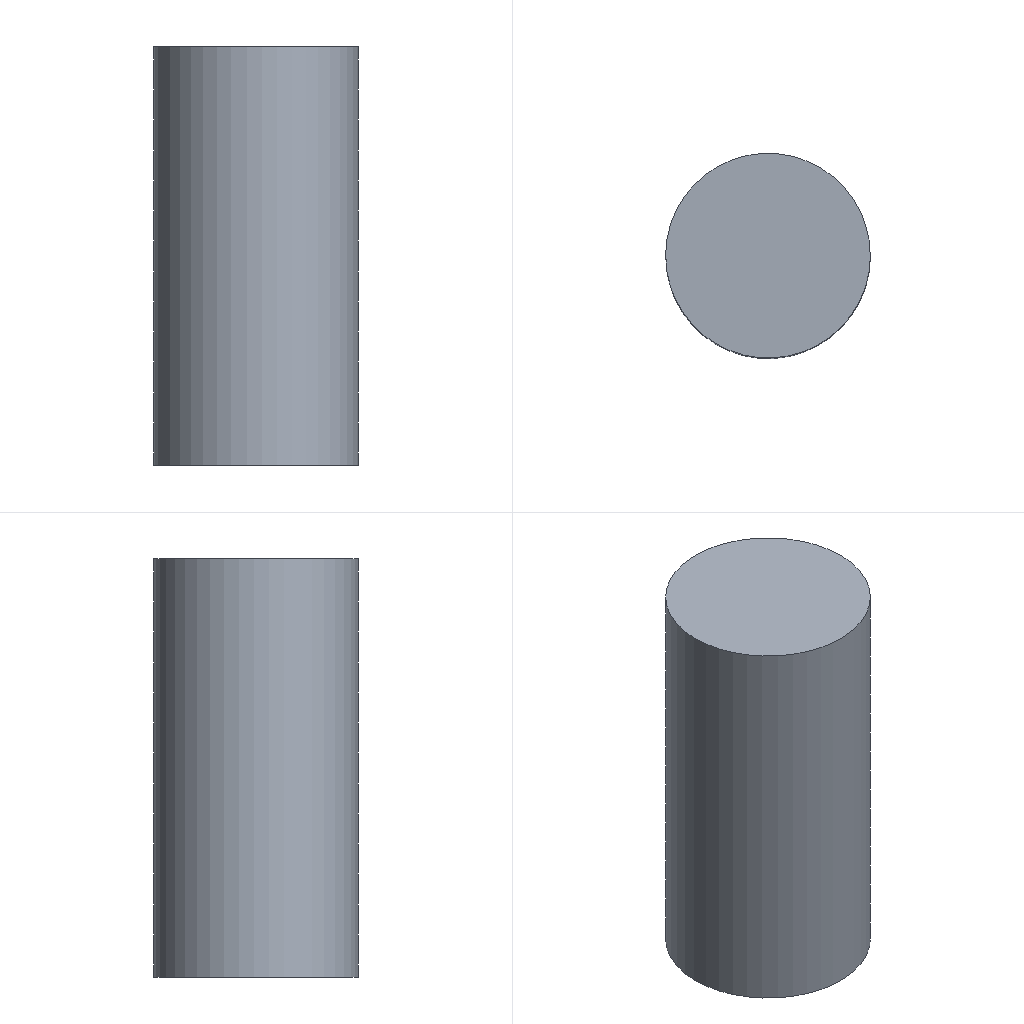Simulation study | abaqus
Set-up summary:
category,name,step,type,value,unit,region
solver,abaqus
solver,version,,,Abaqus/Standard 2020
units,not stated in the deck,,not stated
analysis,deck,,static,static
load_step,Step-1,Step-1,static
load_step,requested,,,1
mesh,nodes,,,29125
mesh,elements,,,72940
element_type,C3D4,,solid,67594
element_type,C3D8R,,solid,5346
load,load commands in deck,,count,2
bc,support commands in deck,,count,5
material,EPS,,in results
material,SOIL,,in results
check,setup vs results,,match,"per instance, exact: element labels, types and connectivity; labels of the nodes the elements use; coordinates of those nodes at SINGLE_PRECISION in 1 of 2 instance(s)"
Abaqus input file, long lists of numbers shortened, first 1042 of 4091 lines:
*Heading
** Job name: Job-1 Model name: Model-1
** Generated by: Abaqus/CAE 2020
*Preprint, echo=NO, model=NO, history=NO, contact=NO
**
** PARTS
**
*Part, name=Parricles
*Node
      1,    12.783,  0.9336,   23.451
      2,    13.63,   4.46,   20.722
** (22963 more lines like these left out)
*Element, type=C3D4
  1, 17460, 17461, 17462, 17463
  2,  2296, 17464, 17465, 17460
** (67592 more lines like these left out)
*Nset, nset=Set-4, generate
     1,  22965,      1
*Elset, elset=Set-4, generate
     1,  67594,      1
*Nset, nset=eps-all, generate
     1,  22965,      1
*Elset, elset=eps-all, generate
     1,  67594,      1
** Section: eps
*Solid Section, elset=Set-4, material=eps
,
*End Part
**
*Part, name=soil
*Node
      1,   15.958,  -11.294,           0.
      2,   18.578,  -6.089,           0.
** (6158 more lines like these left out)
*Element, type=C3D8R
   1,  291,  286,  263,  294,   71,   66,   43,   74
   2,  286,  260,  239,  263,   66,   40,   19,   43
** (5344 more lines like these left out)
*Nset, nset=Set-2, generate
    1,  6160,     1
*Elset, elset=Set-2, generate
    1,  5346,     1
** Section: soil
*Solid Section, elset=Set-2, material=soil
,
*End Part
**
**
** ASSEMBLY
**
*Assembly, name=Assembly
**
*Instance, name=Parricles-1, part=Parricles
       -14.6,        -14.7,           0.
*End Instance
**
*Instance, name=soil-1, part=soil
*End Instance
**
*Nset, nset=Set-1, instance=soil-1, generate
   1,  220,    1
*Elset, elset=Set-1, instance=soil-1, generate
   1,  198,    1
*Nset, nset=Set-2, instance=soil-1, generate
 5941,  6160,     1
*Elset, elset=Set-2, instance=soil-1, generate
 5149,  5346,     1
*Nset, nset=Set-3, instance=soil-1, generate
   1,  220,    1
*Elset, elset=Set-3, instance=soil-1, generate
   1,  198,    1
*Elset, elset=_Surf-1_S4, internal, instance=soil-1
    2,    3,    8,    9,   10,   15,   22,   23,   24,   31,   32,   36,   37,   39,   41,   43
   44,   61,   62,   85,   88,  186,  187,  200,  201,  206,  207,  208,  213,  220,  221,  222
** (37 more lines like these left out)
*Elset, elset=_Surf-1_S6, internal, instance=soil-1
    4,    5,    7,   11,   12,   13,   14,   17,   19,   21,   30,   35,   38,   40,   42,   49
   53,   56,   59,  202,  203,  205,  209,  210,  211,  212,  215,  217,  219,  228,  233,  236
** (31 more lines like these left out)
*Surface, type=ELEMENT, name=Surf-1
_Surf-1_S4, S4
_Surf-1_S6, S6
*Elset, elset=_Surf-2_S1, internal, instance=soil-1, generate
 5149,  5346,     1
*Surface, type=ELEMENT, name=Surf-2
_Surf-2_S1, S1
** Constraint: Constraint-1
*Embedded Element
Parricles-1.eps-all
*Elset, elset=__Int-1_gcs0_1_S4, internal, instance=Parricles-1
  11,  14,  23, 142
*Elset, elset=__Int-1_gcs0_1_S3, internal, instance=Parricles-1
  30,  39,  43,  47,  49,  50,  52,  62,  75,  77,  80,  85,  87,  88,  89,  90
  92,  93,  97,  98, 100, 101, 103, 104, 105, 106, 107, 108, 109, 110, 111, 112
** (2 more lines like these left out)
*Elset, elset=__Int-1_gcs0_1_S1, internal, instance=Parricles-1
 74,
*Elset, elset=__Int-1_gcs0_1_S2, internal, instance=Parricles-1
  86,  91,  96, 102, 141, 147
*Surface, type=ELEMENT, name=_Int-1_gcs0_1, internal
__Int-1_gcs0_1_S4, S4
__Int-1_gcs0_1_S3, S3
__Int-1_gcs0_1_S2, S2
__Int-1_gcs0_1_S1, S1
*Elset, elset=__Int-1_gcs0_2_S3, internal, instance=Parricles-1
 162, 187, 193, 196, 199, 200, 204, 213, 214, 215, 216, 217, 218, 219, 220, 222
 223, 226, 232, 233, 234, 236, 237, 238, 239, 241, 242, 243, 244, 245, 246, 247
** (2 more lines like these left out)
*Elset, elset=__Int-1_gcs0_2_S4, internal, instance=Parricles-1
 174, 212, 235, 255
*Elset, elset=__Int-1_gcs0_2_S1, internal, instance=Parricles-1
 224,
*Elset, elset=__Int-1_gcs0_2_S2, internal, instance=Parricles-1
 225, 227, 231, 260, 271, 284
*Surface, type=ELEMENT, name=_Int-1_gcs0_2, internal
__Int-1_gcs0_2_S3, S3
__Int-1_gcs0_2_S4, S4
__Int-1_gcs0_2_S2, S2
__Int-1_gcs0_2_S1, S1
*Elset, elset=__Int-1_gcs0_3_S3, internal, instance=Parricles-1
 304, 310, 322, 323, 328, 334, 340, 361, 362, 363, 365, 366, 367, 369, 370, 371
 375, 376, 377, 379, 380, 381, 382, 383, 384, 385, 387, 388, 389, 390, 391, 392
** (3 more lines like these left out)
*Elset, elset=__Int-1_gcs0_3_S2, internal, instance=Parricles-1
 306, 437
*Elset, elset=__Int-1_gcs0_3_S4, internal, instance=Parricles-1
 330,
*Elset, elset=__Int-1_gcs0_3_S1, internal, instance=Parricles-1
 431,
*Surface, type=ELEMENT, name=_Int-1_gcs0_3, internal
__Int-1_gcs0_3_S3, S3
__Int-1_gcs0_3_S2, S2
__Int-1_gcs0_3_S4, S4
__Int-1_gcs0_3_S1, S1
*Elset, elset=__Int-1_gcs0_4_S1, internal, instance=Parricles-1
 495, 524, 598
*Elset, elset=__Int-1_gcs0_4_S4, internal, instance=Parricles-1
 500, 502, 560, 586
*Elset, elset=__Int-1_gcs0_4_S3, internal, instance=Parricles-1
 509, 515, 530, 531, 532, 533, 535, 536, 537, 539, 542, 543, 544, 545, 546, 547
 548, 551, 552, 555, 556, 557, 558, 559, 561, 562, 563, 564, 566, 567, 569, 570
** (2 more lines like these left out)
*Elset, elset=__Int-1_gcs0_4_S2, internal, instance=Parricles-1
 550, 610
*Surface, type=ELEMENT, name=_Int-1_gcs0_4, internal
__Int-1_gcs0_4_S1, S1
__Int-1_gcs0_4_S4, S4
__Int-1_gcs0_4_S2, S2
__Int-1_gcs0_4_S3, S3
*Elset, elset=__Int-1_gcs0_5_S4, internal, instance=Parricles-1
 618, 633, 712
*Elset, elset=__Int-1_gcs0_5_S3, internal, instance=Parricles-1
 620, 623, 626, 644, 648, 666, 677, 679, 680, 681, 682, 683, 684, 685, 687, 689
 690, 691, 692, 693, 694, 695, 696, 697, 698, 699, 701, 702, 703, 704, 705, 708
** (2 more lines like these left out)
*Elset, elset=__Int-1_gcs0_5_S1, internal, instance=Parricles-1
 650,
*Elset, elset=__Int-1_gcs0_5_S2, internal, instance=Parricles-1
 678,
*Surface, type=ELEMENT, name=_Int-1_gcs0_5, internal
__Int-1_gcs0_5_S4, S4
__Int-1_gcs0_5_S3, S3
__Int-1_gcs0_5_S2, S2
__Int-1_gcs0_5_S1, S1
*Elset, elset=__Int-1_gcs0_6_S3, internal, instance=Parricles-1
 765, 770, 819, 823, 829, 832, 833, 834, 835, 837, 839, 840, 841, 842, 843, 846
 847, 850, 851, 852, 854, 856, 858, 859, 860, 861, 862, 863, 864, 865, 866, 868
** (2 more lines like these left out)
*Elset, elset=__Int-1_gcs0_6_S4, internal, instance=Parricles-1
 792, 826, 828, 838, 844, 867, 888, 902
*Elset, elset=__Int-1_gcs0_6_S1, internal, instance=Parricles-1
 796,
*Elset, elset=__Int-1_gcs0_6_S2, internal, instance=Parricles-1
 845, 896, 903
*Surface, type=ELEMENT, name=_Int-1_gcs0_6, internal
__Int-1_gcs0_6_S3, S3
__Int-1_gcs0_6_S4, S4
__Int-1_gcs0_6_S2, S2
__Int-1_gcs0_6_S1, S1
*Elset, elset=__Int-1_gcs0_7_S3, internal, instance=Parricles-1
  931,  962,  964,  985,  986,  987,  988,  989,  990,  991,  992,  993,  994,  996,  997, 1000
 1001, 1003, 1004, 1005, 1006, 1009, 1011, 1012, 1014, 1015, 1016, 1017, 1018, 1019, 1020, 1021
** (3 more lines like these left out)
*Elset, elset=__Int-1_gcs0_7_S4, internal, instance=Parricles-1
 954, 961
*Elset, elset=__Int-1_gcs0_7_S2, internal, instance=Parricles-1
  995, 1008, 1022, 1054
*Surface, type=ELEMENT, name=_Int-1_gcs0_7, internal
__Int-1_gcs0_7_S3, S3
__Int-1_gcs0_7_S4, S4
__Int-1_gcs0_7_S2, S2
*Elset, elset=__Int-1_gcs0_8_S3, internal, instance=Parricles-1
 1071, 1075, 1079, 1083, 1090, 1113, 1121, 1130, 1131, 1133, 1134, 1136, 1137, 1138, 1139, 1140
 1142, 1145, 1148, 1149, 1150, 1152, 1153, 1154, 1155, 1156, 1157, 1158, 1159, 1161, 1162, 1163
** (2 more lines like these left out)
*Elset, elset=__Int-1_gcs0_8_S2, internal, instance=Parricles-1
 1086, 1151, 1165
*Elset, elset=__Int-1_gcs0_8_S1, internal, instance=Parricles-1
 1116, 1166, 1182
*Elset, elset=__Int-1_gcs0_8_S4, internal, instance=Parricles-1
 1144, 1194
*Surface, type=ELEMENT, name=_Int-1_gcs0_8, internal
__Int-1_gcs0_8_S3, S3
__Int-1_gcs0_8_S2, S2
__Int-1_gcs0_8_S4, S4
__Int-1_gcs0_8_S1, S1
*Elset, elset=__Int-1_gcs0_9_S4, internal, instance=Parricles-1
 1217, 1300
*Elset, elset=__Int-1_gcs0_9_S3, internal, instance=Parricles-1
 1230, 1234, 1248, 1269, 1272, 1273, 1275, 1276, 1277, 1280, 1282, 1283, 1284, 1285, 1287, 1288
 1289, 1290, 1291, 1292, 1293, 1294, 1295, 1297, 1299, 1303, 1304, 1306, 1307, 1308, 1309, 1310
** (2 more lines like these left out)
*Elset, elset=__Int-1_gcs0_9_S2, internal, instance=Parricles-1
 1252, 1253, 1298, 1305, 1311, 1338
*Surface, type=ELEMENT, name=_Int-1_gcs0_9, internal
__Int-1_gcs0_9_S4, S4
__Int-1_gcs0_9_S3, S3
__Int-1_gcs0_9_S2, S2
*Elset, elset=__Int-1_gcs0_10_S3, internal, instance=Parricles-1
 1346, 1348, 1362, 1363, 1367, 1368, 1373, 1378, 1394, 1403, 1404, 1405, 1406, 1407, 1408, 1409
 1410, 1411, 1412, 1414, 1415, 1416, 1417, 1419, 1422, 1424, 1425, 1426, 1427, 1428, 1430, 1431
** (2 more lines like these left out)
*Elset, elset=__Int-1_gcs0_10_S1, internal, instance=Parricles-1
 1350, 1361, 1472
*Elset, elset=__Int-1_gcs0_10_S2, internal, instance=Parricles-1
 1351, 1354
*Elset, elset=__Int-1_gcs0_10_S4, internal, instance=Parricles-1
 1389, 1436, 1459
*Surface, type=ELEMENT, name=_Int-1_gcs0_10, internal
__Int-1_gcs0_10_S3, S3
__Int-1_gcs0_10_S1, S1
__Int-1_gcs0_10_S2, S2
__Int-1_gcs0_10_S4, S4
*Elset, elset=__Int-1_gcs0_11_S2, internal, instance=Parricles-1
 1479, 1544, 1568, 1603, 1605, 1608
*Elset, elset=__Int-1_gcs0_11_S3, internal, instance=Parricles-1
 1487, 1501, 1524, 1530, 1539, 1541, 1542, 1545, 1560, 1564, 1565, 1566, 1567, 1569, 1570, 1571
 1572, 1573, 1574, 1575, 1576, 1577, 1579, 1580, 1581, 1582, 1584, 1588, 1589, 1590, 1592, 1594
** (2 more lines like these left out)
*Elset, elset=__Int-1_gcs0_11_S1, internal, instance=Parricles-1
 1552,
*Elset, elset=__Int-1_gcs0_11_S4, internal, instance=Parricles-1
 1585, 1593
*Surface, type=ELEMENT, name=_Int-1_gcs0_11, internal
__Int-1_gcs0_11_S2, S2
__Int-1_gcs0_11_S3, S3
__Int-1_gcs0_11_S4, S4
__Int-1_gcs0_11_S1, S1
*Elset, elset=__Int-1_gcs0_12_S2, internal, instance=Parricles-1
 1637, 1703, 1733, 1735, 1750, 1762
*Elset, elset=__Int-1_gcs0_12_S3, internal, instance=Parricles-1
 1650, 1653, 1655, 1682, 1689, 1705, 1706, 1707, 1708, 1709, 1711, 1712, 1713, 1714, 1715, 1717
 1718, 1719, 1720, 1721, 1723, 1724, 1725, 1726, 1727, 1728, 1729, 1731, 1734, 1737, 1739, 1740
** (2 more lines like these left out)
*Elset, elset=__Int-1_gcs0_12_S1, internal, instance=Parricles-1
 1656, 1680
*Elset, elset=__Int-1_gcs0_12_S4, internal, instance=Parricles-1
 1688, 1704, 1730
*Surface, type=ELEMENT, name=_Int-1_gcs0_12, internal
__Int-1_gcs0_12_S2, S2
__Int-1_gcs0_12_S3, S3
__Int-1_gcs0_12_S4, S4
__Int-1_gcs0_12_S1, S1
*Elset, elset=__Int-1_gcs0_13_S2, internal, instance=Parricles-1
 1780, 1849, 1860, 1910, 1927
*Elset, elset=__Int-1_gcs0_13_S4, internal, instance=Parricles-1
 1784, 1796, 1822, 1867, 1887, 1903
*Elset, elset=__Int-1_gcs0_13_S3, internal, instance=Parricles-1
 1791, 1795, 1803, 1811, 1819, 1846, 1851, 1861, 1863, 1864, 1866, 1868, 1869, 1870, 1872, 1877
 1878, 1880, 1883, 1884, 1885, 1886, 1888, 1889, 1890, 1891, 1892, 1893, 1894, 1895, 1896, 1897
** (3 more lines like these left out)
*Surface, type=ELEMENT, name=_Int-1_gcs0_13, internal
__Int-1_gcs0_13_S2, S2
__Int-1_gcs0_13_S4, S4
__Int-1_gcs0_13_S3, S3
*Elset, elset=__Int-1_gcs0_14_S3, internal, instance=Parricles-1
 1947, 1955, 1973, 1975, 1980, 1991, 1997, 2007, 2028, 2032, 2033, 2034, 2035, 2036, 2037, 2039
 2041, 2042, 2043, 2044, 2045, 2050, 2051, 2052, 2055, 2056, 2057, 2058, 2059, 2060, 2062, 2064
** (2 more lines like these left out)
*Elset, elset=__Int-1_gcs0_14_S1, internal, instance=Parricles-1
 1953, 1956, 1958, 2002
*Elset, elset=__Int-1_gcs0_14_S4, internal, instance=Parricles-1
 1961, 1988, 2011, 2061
*Elset, elset=__Int-1_gcs0_14_S2, internal, instance=Parricles-1
 2017, 2084, 2085, 2100
*Surface, type=ELEMENT, name=_Int-1_gcs0_14, internal
__Int-1_gcs0_14_S3, S3
__Int-1_gcs0_14_S1, S1
__Int-1_gcs0_14_S4, S4
__Int-1_gcs0_14_S2, S2
*Elset, elset=__Int-1_gcs0_15_S4, internal, instance=Parricles-1
 2126, 2147
*Elset, elset=__Int-1_gcs0_15_S3, internal, instance=Parricles-1
 2135, 2144, 2145, 2151, 2164, 2170, 2172, 2174, 2178, 2180, 2181, 2182, 2183, 2184, 2185, 2188
 2189, 2190, 2191, 2194, 2195, 2196, 2197, 2198, 2199, 2200, 2201, 2202, 2203, 2204, 2205, 2206
** (2 more lines like these left out)
*Elset, elset=__Int-1_gcs0_15_S1, internal, instance=Parricles-1
 2161, 2166, 2235
*Elset, elset=__Int-1_gcs0_15_S2, internal, instance=Parricles-1
 2192, 2193, 2228, 2234, 2236
*Surface, type=ELEMENT, name=_Int-1_gcs0_15, internal
__Int-1_gcs0_15_S4, S4
__Int-1_gcs0_15_S3, S3
__Int-1_gcs0_15_S2, S2
__Int-1_gcs0_15_S1, S1
*Elset, elset=__Int-1_gcs0_16_S3, internal, instance=Parricles-1
 2249, 2258, 2269, 2298, 2305, 2309, 2311, 2313, 2315, 2316, 2317, 2318, 2319, 2321, 2322, 2323
 2324, 2327, 2328, 2329, 2330, 2332, 2333, 2334, 2335, 2337, 2338, 2339, 2341, 2342, 2343, 2344
** (2 more lines like these left out)
*Elset, elset=__Int-1_gcs0_16_S2, internal, instance=Parricles-1
 2250, 2314, 2340, 2350, 2354, 2356, 2369
*Elset, elset=__Int-1_gcs0_16_S4, internal, instance=Parricles-1
 2325, 2371
*Surface, type=ELEMENT, name=_Int-1_gcs0_16, internal
__Int-1_gcs0_16_S3, S3
__Int-1_gcs0_16_S2, S2
__Int-1_gcs0_16_S4, S4
*Elset, elset=__Int-1_gcs0_17_S3, internal, instance=Parricles-1
 2384, 2395, 2402, 2404, 2418, 2425, 2427, 2433, 2449, 2451, 2455, 2456, 2457, 2458, 2459, 2460
 2461, 2462, 2463, 2464, 2465, 2466, 2468, 2469, 2470, 2471, 2472, 2473, 2474, 2475, 2476, 2477
** (2 more lines like these left out)
*Elset, elset=__Int-1_gcs0_17_S4, internal, instance=Parricles-1
 2399, 2419, 2448, 2452
*Elset, elset=__Int-1_gcs0_17_S1, internal, instance=Parricles-1
 2420,
*Elset, elset=__Int-1_gcs0_17_S2, internal, instance=Parricles-1
 2453, 2491, 2508, 2511, 2517
*Surface, type=ELEMENT, name=_Int-1_gcs0_17, internal
__Int-1_gcs0_17_S3, S3
__Int-1_gcs0_17_S4, S4
__Int-1_gcs0_17_S2, S2
__Int-1_gcs0_17_S1, S1
*Elset, elset=__Int-1_gcs0_18_S3, internal, instance=Parricles-1
 2533, 2568, 2569, 2576, 2578, 2579, 2580, 2582, 2583, 2588, 2590, 2591, 2593, 2594, 2596, 2597
 2600, 2601, 2602, 2603, 2605, 2606, 2607, 2608, 2609, 2611, 2612, 2614, 2615, 2616, 2617, 2618
** (2 more lines like these left out)
*Elset, elset=__Int-1_gcs0_18_S1, internal, instance=Parricles-1
 2541, 2560, 2563
*Elset, elset=__Int-1_gcs0_18_S2, internal, instance=Parricles-1
 2543, 2565, 2585, 2640, 2641, 2643
*Elset, elset=__Int-1_gcs0_18_S4, internal, instance=Parricles-1
 2573, 2598, 2613, 2620
*Surface, type=ELEMENT, name=_Int-1_gcs0_18, internal
__Int-1_gcs0_18_S3, S3
__Int-1_gcs0_18_S1, S1
__Int-1_gcs0_18_S2, S2
__Int-1_gcs0_18_S4, S4
*Elset, elset=__Int-1_gcs0_19_S3, internal, instance=Parricles-1
 2664, 2666, 2669, 2684, 2691, 2695, 2696, 2697, 2698, 2699, 2700, 2701, 2702, 2703, 2704, 2708
 2709, 2711, 2712, 2714, 2715, 2716, 2717, 2718, 2720, 2721, 2722, 2723, 2724, 2726, 2727, 2728
** (3 more lines like these left out)
*Elset, elset=__Int-1_gcs0_19_S4, internal, instance=Parricles-1
 2671,
*Elset, elset=__Int-1_gcs0_19_S2, internal, instance=Parricles-1
 2705, 2732
*Surface, type=ELEMENT, name=_Int-1_gcs0_19, internal
__Int-1_gcs0_19_S3, S3
__Int-1_gcs0_19_S4, S4
__Int-1_gcs0_19_S2, S2
*Elset, elset=__Int-1_gcs0_20_S4, internal, instance=Parricles-1
 2788, 2812, 2838
*Elset, elset=__Int-1_gcs0_20_S3, internal, instance=Parricles-1
 2796, 2823, 2848, 2860, 2875, 2877, 2878, 2879, 2880, 2881, 2884, 2885, 2887, 2889, 2890, 2891
 2893, 2895, 2896, 2897, 2898, 2899, 2900, 2901, 2903, 2904, 2905, 2906, 2907, 2908, 2910, 2911
** (3 more lines like these left out)
*Elset, elset=__Int-1_gcs0_20_S2, internal, instance=Parricles-1
 2902,
*Surface, type=ELEMENT, name=_Int-1_gcs0_20, internal
__Int-1_gcs0_20_S4, S4
__Int-1_gcs0_20_S3, S3
__Int-1_gcs0_20_S2, S2
*Elset, elset=__Int-1_gcs0_21_S1, internal, instance=Parricles-1
 2964, 2984
*Elset, elset=__Int-1_gcs0_21_S3, internal, instance=Parricles-1
 2967, 2970, 2980, 2983, 2987, 2995, 3012, 3013, 3042, 3047, 3048, 3049, 3050, 3051, 3052, 3053
 3054, 3055, 3056, 3058, 3060, 3062, 3063, 3065, 3067, 3068, 3069, 3070, 3071, 3072, 3073, 3074
** (3 more lines like these left out)
*Elset, elset=__Int-1_gcs0_21_S4, internal, instance=Parricles-1
 3008, 3080
*Elset, elset=__Int-1_gcs0_21_S2, internal, instance=Parricles-1
 3057, 3103
*Surface, type=ELEMENT, name=_Int-1_gcs0_21, internal
__Int-1_gcs0_21_S1, S1
__Int-1_gcs0_21_S3, S3
__Int-1_gcs0_21_S4, S4
__Int-1_gcs0_21_S2, S2
*Elset, elset=__Int-1_gcs0_22_S3, internal, instance=Parricles-1
 3126, 3146, 3149, 3151, 3168, 3170, 3171, 3180, 3184, 3195, 3196, 3197, 3199, 3202, 3205, 3206
 3207, 3208, 3211, 3212, 3214, 3215, 3216, 3217, 3219, 3220, 3221, 3222, 3223, 3224, 3225, 3227
** (2 more lines like these left out)
*Elset, elset=__Int-1_gcs0_22_S4, internal, instance=Parricles-1
 3135, 3159, 3172, 3204, 3251, 3260
*Elset, elset=__Int-1_gcs0_22_S2, internal, instance=Parricles-1
 3189, 3198, 3210, 3231
*Surface, type=ELEMENT, name=_Int-1_gcs0_22, internal
__Int-1_gcs0_22_S3, S3
__Int-1_gcs0_22_S4, S4
__Int-1_gcs0_22_S2, S2
*Elset, elset=__Int-1_gcs0_23_S4, internal, instance=Parricles-1
 3271, 3284, 3294
*Elset, elset=__Int-1_gcs0_23_S3, internal, instance=Parricles-1
 3285, 3290, 3295, 3301, 3314, 3316, 3319, 3320, 3322, 3323, 3324, 3325, 3326, 3327, 3328, 3329
 3330, 3331, 3332, 3333, 3334, 3336, 3337, 3338, 3339, 3340, 3342, 3343, 3344, 3345, 3347, 3348
** (3 more lines like these left out)
*Elset, elset=__Int-1_gcs0_23_S2, internal, instance=Parricles-1
 3371, 3382, 3384
*Elset, elset=__Int-1_gcs0_23_S1, internal, instance=Parricles-1
 3376,
*Surface, type=ELEMENT, name=_Int-1_gcs0_23, internal
__Int-1_gcs0_23_S4, S4
__Int-1_gcs0_23_S3, S3
__Int-1_gcs0_23_S2, S2
__Int-1_gcs0_23_S1, S1
*Elset, elset=__Int-1_gcs0_24_S3, internal, instance=Parricles-1
 3394, 3409, 3421, 3432, 3436, 3443, 3444, 3445, 3446, 3448, 3450, 3451, 3455, 3456, 3457, 3458
 3459, 3460, 3461, 3462, 3464, 3465, 3466, 3467, 3468, 3469, 3470, 3471, 3473, 3474, 3475, 3476
** (2 more lines like these left out)
*Elset, elset=__Int-1_gcs0_24_S4, internal, instance=Parricles-1
 3399, 3425, 3447
*Elset, elset=__Int-1_gcs0_24_S1, internal, instance=Parricles-1
 3430,
*Elset, elset=__Int-1_gcs0_24_S2, internal, instance=Parricles-1
 3449, 3472, 3492
*Surface, type=ELEMENT, name=_Int-1_gcs0_24, internal
__Int-1_gcs0_24_S3, S3
__Int-1_gcs0_24_S4, S4
__Int-1_gcs0_24_S2, S2
__Int-1_gcs0_24_S1, S1
*Elset, elset=__Int-1_gcs0_25_S3, internal, instance=Parricles-1
 3525, 3553, 3556, 3567, 3569, 3570, 3571, 3573, 3574, 3575, 3576, 3577, 3578, 3580, 3582, 3583
 3584, 3585, 3586, 3588, 3589, 3590, 3591, 3592, 3593, 3594, 3595, 3596, 3598, 3599, 3600, 3601
** (3 more lines like these left out)
*Elset, elset=__Int-1_gcs0_25_S4, internal, instance=Parricles-1
 3529, 3536, 3572
*Elset, elset=__Int-1_gcs0_25_S2, internal, instance=Parricles-1
 3579, 3581, 3587, 3613
*Surface, type=ELEMENT, name=_Int-1_gcs0_25, internal
__Int-1_gcs0_25_S3, S3
__Int-1_gcs0_25_S4, S4
__Int-1_gcs0_25_S2, S2
*Elset, elset=__Int-1_gcs0_26_S1, internal, instance=Parricles-1
 3644, 3679
*Elset, elset=__Int-1_gcs0_26_S3, internal, instance=Parricles-1
 3654, 3664, 3666, 3672, 3688, 3690, 3693, 3699, 3700, 3702, 3703, 3704, 3706, 3707, 3708, 3710
 3711, 3716, 3717, 3718, 3723, 3725, 3728, 3730, 3731, 3734, 3735, 3736, 3737, 3738, 3739, 3741
** (2 more lines like these left out)
*Elset, elset=__Int-1_gcs0_26_S4, internal, instance=Parricles-1
 3659, 3674, 3677, 3685, 3713
*Elset, elset=__Int-1_gcs0_26_S2, internal, instance=Parricles-1
 3712, 3715, 3733, 3744, 3755, 3768
*Surface, type=ELEMENT, name=_Int-1_gcs0_26, internal
__Int-1_gcs0_26_S1, S1
__Int-1_gcs0_26_S3, S3
__Int-1_gcs0_26_S4, S4
__Int-1_gcs0_26_S2, S2
*Elset, elset=__Int-1_gcs0_27_S3, internal, instance=Parricles-1
 3782, 3785, 3843, 3844, 3849, 3857, 3858, 3859, 3860, 3861, 3862, 3863, 3864, 3866, 3867, 3868
 3869, 3871, 3874, 3875, 3877, 3878, 3879, 3880, 3882, 3883, 3885, 3886, 3887, 3891, 3892, 3893
** (3 more lines like these left out)
*Elset, elset=__Int-1_gcs0_27_S4, internal, instance=Parricles-1
 3784, 3827, 3926, 3940
*Elset, elset=__Int-1_gcs0_27_S2, internal, instance=Parricles-1
 3870, 3888, 3902
*Surface, type=ELEMENT, name=_Int-1_gcs0_27, internal
__Int-1_gcs0_27_S3, S3
__Int-1_gcs0_27_S4, S4
__Int-1_gcs0_27_S2, S2
*Elset, elset=__Int-1_gcs0_28_S3, internal, instance=Parricles-1
 3944, 3970, 3977, 3995, 4012, 4013, 4014, 4015, 4016, 4017, 4018, 4019, 4020, 4022, 4023, 4026
 4027, 4028, 4029, 4030, 4031, 4032, 4033, 4034, 4035, 4037, 4038, 4039, 4040, 4041, 4042, 4043
** (2 more lines like these left out)
*Elset, elset=__Int-1_gcs0_28_S4, internal, instance=Parricles-1
 3954,
*Elset, elset=__Int-1_gcs0_28_S1, internal, instance=Parricles-1
 3967, 3978, 3979, 3980, 3984
*Elset, elset=__Int-1_gcs0_28_S2, internal, instance=Parricles-1
 4024, 4025, 4036, 4051, 4069
*Surface, type=ELEMENT, name=_Int-1_gcs0_28, internal
__Int-1_gcs0_28_S3, S3
__Int-1_gcs0_28_S4, S4
__Int-1_gcs0_28_S2, S2
__Int-1_gcs0_28_S1, S1
*Elset, elset=__Int-1_gcs0_29_S4, internal, instance=Parricles-1
 4088, 4108, 4115, 4124, 4157, 4171, 4194
*Elset, elset=__Int-1_gcs0_29_S3, internal, instance=Parricles-1
 4092, 4100, 4114, 4131, 4133, 4147, 4151, 4153, 4154, 4155, 4156, 4163, 4164, 4168, 4170, 4173
 4174, 4175, 4176, 4177, 4178, 4179, 4182, 4185, 4186, 4188, 4189, 4190, 4191, 4192, 4193, 4195
** (2 more lines like these left out)
*Elset, elset=__Int-1_gcs0_29_S1, internal, instance=Parricles-1
 4134, 4169
*Elset, elset=__Int-1_gcs0_29_S2, internal, instance=Parricles-1
 4160, 4184, 4219, 4229
*Surface, type=ELEMENT, name=_Int-1_gcs0_29, internal
__Int-1_gcs0_29_S4, S4
__Int-1_gcs0_29_S3, S3
__Int-1_gcs0_29_S2, S2
__Int-1_gcs0_29_S1, S1
*Elset, elset=__Int-1_gcs0_30_S4, internal, instance=Parricles-1
 4233, 4241, 4273
*Elset, elset=__Int-1_gcs0_30_S3, internal, instance=Parricles-1
 4238, 4263, 4266, 4289, 4300, 4301, 4302, 4303, 4304, 4305, 4306, 4307, 4308, 4309, 4310, 4311
 4314, 4315, 4316, 4318, 4319, 4321, 4322, 4324, 4325, 4327, 4328, 4329, 4330, 4331, 4332, 4333
** (3 more lines like these left out)
*Elset, elset=__Int-1_gcs0_30_S1, internal, instance=Parricles-1
 4269,
*Elset, elset=__Int-1_gcs0_30_S2, internal, instance=Parricles-1
 4297, 4352
*Surface, type=ELEMENT, name=_Int-1_gcs0_30, internal
__Int-1_gcs0_30_S4, S4
__Int-1_gcs0_30_S3, S3
__Int-1_gcs0_30_S2, S2
__Int-1_gcs0_30_S1, S1
*Elset, elset=__Int-1_gcs0_31_S3, internal, instance=Parricles-1
 4385, 4403, 4413, 4419, 4433, 4434, 4439, 4449, 4451, 4467, 4469, 4470, 4471, 4472, 4473, 4474
 4476, 4478, 4479, 4480, 4481, 4482, 4483, 4484, 4485, 4486, 4488, 4489, 4491, 4495, 4496, 4497
** (2 more lines like these left out)
*Elset, elset=__Int-1_gcs0_31_S1, internal, instance=Parricles-1
 4396,
*Elset, elset=__Int-1_gcs0_31_S4, internal, instance=Parricles-1
 4414, 4465, 4492, 4501
*Elset, elset=__Int-1_gcs0_31_S2, internal, instance=Parricles-1
 4468, 4475, 4487, 4490, 4517
*Surface, type=ELEMENT, name=_Int-1_gcs0_31, internal
__Int-1_gcs0_31_S3, S3
__Int-1_gcs0_31_S1, S1
__Int-1_gcs0_31_S4, S4
__Int-1_gcs0_31_S2, S2
*Elset, elset=__Int-1_gcs0_32_S3, internal, instance=Parricles-1
 4552, 4553, 4574, 4579, 4581, 4605, 4606, 4608, 4610, 4611, 4612, 4613, 4615, 4616, 4619, 4622
 4623, 4624, 4625, 4626, 4627, 4628, 4629, 4630, 4631, 4633, 4634, 4635, 4636, 4638, 4639, 4640
** (3 more lines like these left out)
*Elset, elset=__Int-1_gcs0_32_S4, internal, instance=Parricles-1
 4557,
*Elset, elset=__Int-1_gcs0_32_S1, internal, instance=Parricles-1
 4587, 4658
*Elset, elset=__Int-1_gcs0_32_S2, internal, instance=Parricles-1
 4632, 4662
*Surface, type=ELEMENT, name=_Int-1_gcs0_32, internal
__Int-1_gcs0_32_S3, S3
__Int-1_gcs0_32_S4, S4
__Int-1_gcs0_32_S2, S2
__Int-1_gcs0_32_S1, S1
*Elset, elset=__Int-1_gcs0_33_S3, internal, instance=Parricles-1
 4696, 4714, 4720, 4739, 4758, 4759, 4760, 4763, 4766, 4767, 4769, 4771, 4773, 4774, 4775, 4776
 4778, 4779, 4781, 4783, 4784, 4785, 4787, 4788, 4791, 4792, 4793, 4794, 4795, 4796, 4798, 4800
** (3 more lines like these left out)
*Elset, elset=__Int-1_gcs0_33_S4, internal, instance=Parricles-1
 4699, 4733, 4742
*Elset, elset=__Int-1_gcs0_33_S2, internal, instance=Parricles-1
 4740, 4762, 4764, 4772, 4786, 4809
*Elset, elset=__Int-1_gcs0_33_S1, internal, instance=Parricles-1
 4741, 4805
*Surface, type=ELEMENT, name=_Int-1_gcs0_33, internal
__Int-1_gcs0_33_S3, S3
__Int-1_gcs0_33_S4, S4
__Int-1_gcs0_33_S2, S2
__Int-1_gcs0_33_S1, S1
*Elset, elset=__Int-1_gcs0_34_S4, internal, instance=Parricles-1
 4853, 4855, 4873, 4887, 4901, 4927, 4976, 4982
*Elset, elset=__Int-1_gcs0_34_S3, internal, instance=Parricles-1
 4899, 4906, 4907, 4908, 4909, 4910, 4911, 4913, 4914, 4915, 4916, 4917, 4918, 4919, 4920, 4922
 4923, 4924, 4925, 4926, 4928, 4930, 4931, 4934, 4935, 4937, 4938, 4939, 4942, 4944, 4945, 4947
** (2 more lines like these left out)
*Elset, elset=__Int-1_gcs0_34_S2, internal, instance=Parricles-1
 4941,
*Surface, type=ELEMENT, name=_Int-1_gcs0_34, internal
__Int-1_gcs0_34_S4, S4
__Int-1_gcs0_34_S3, S3
__Int-1_gcs0_34_S2, S2
*Elset, elset=__Int-1_gcs0_35_S4, internal, instance=Parricles-1
 4991, 5030, 5078, 5090, 5118
*Elset, elset=__Int-1_gcs0_35_S1, internal, instance=Parricles-1
 4998, 5108
*Elset, elset=__Int-1_gcs0_35_S3, internal, instance=Parricles-1
 4999, 5015, 5035, 5052, 5054, 5055, 5056, 5058, 5059, 5061, 5062, 5063, 5064, 5065, 5067, 5068
 5069, 5070, 5071, 5072, 5073, 5076, 5079, 5080, 5081, 5082, 5085, 5086, 5087, 5088, 5089, 5093
** (3 more lines like these left out)
*Elset, elset=__Int-1_gcs0_35_S2, internal, instance=Parricles-1
 5092,
*Surface, type=ELEMENT, name=_Int-1_gcs0_35, internal
__Int-1_gcs0_35_S4, S4
__Int-1_gcs0_35_S1, S1
__Int-1_gcs0_35_S2, S2
__Int-1_gcs0_35_S3, S3
*Elset, elset=__Int-1_gcs0_36_S3, internal, instance=Parricles-1
 5148, 5156, 5157, 5170, 5174, 5180, 5182, 5188, 5208, 5210, 5211, 5213, 5232, 5233, 5234, 5235
 5236, 5237, 5238, 5239, 5240, 5241, 5242, 5243, 5244, 5246, 5247, 5248, 5249, 5250, 5251, 5253
** (2 more lines like these left out)
*Elset, elset=__Int-1_gcs0_36_S4, internal, instance=Parricles-1
 5153, 5155, 5194, 5258, 5261, 5291, 5292
*Elset, elset=__Int-1_gcs0_36_S2, internal, instance=Parricles-1
 5163, 5259, 5277
*Elset, elset=__Int-1_gcs0_36_S1, internal, instance=Parricles-1
 5175, 5299
*Surface, type=ELEMENT, name=_Int-1_gcs0_36, internal
__Int-1_gcs0_36_S3, S3
__Int-1_gcs0_36_S4, S4
__Int-1_gcs0_36_S2, S2
__Int-1_gcs0_36_S1, S1
*Elset, elset=__Int-1_gcs0_37_S4, internal, instance=Parricles-1
 5302, 5305, 5324, 5338, 5357, 5403
*Elset, elset=__Int-1_gcs0_37_S3, internal, instance=Parricles-1
 5308, 5319, 5330, 5333, 5361, 5364, 5365, 5367, 5369, 5370, 5371, 5372, 5374, 5375, 5376, 5378
 5379, 5380, 5381, 5382, 5383, 5385, 5386, 5387, 5388, 5389, 5390, 5391, 5393, 5394, 5396, 5397
** (2 more lines like these left out)
*Elset, elset=__Int-1_gcs0_37_S1, internal, instance=Parricles-1
 5316,
*Elset, elset=__Int-1_gcs0_37_S2, internal, instance=Parricles-1
 5423,
*Surface, type=ELEMENT, name=_Int-1_gcs0_37, internal
__Int-1_gcs0_37_S4, S4
__Int-1_gcs0_37_S3, S3
__Int-1_gcs0_37_S2, S2
__Int-1_gcs0_37_S1, S1
*Elset, elset=__Int-1_gcs0_38_S3, internal, instance=Parricles-1
 5447, 5473, 5478, 5481, 5493, 5494, 5495, 5509, 5510, 5511, 5513, 5514, 5516, 5517, 5518, 5519
 5522, 5523, 5524, 5525, 5526, 5527, 5530, 5531, 5532, 5534, 5535, 5536, 5537, 5538, 5539, 5541
** (2 more lines like these left out)
*Elset, elset=__Int-1_gcs0_38_S2, internal, instance=Parricles-1
 5461, 5512, 5549, 5554
*Elset, elset=__Int-1_gcs0_38_S4, internal, instance=Parricles-1
 5501, 5506, 5521, 5569
*Surface, type=ELEMENT, name=_Int-1_gcs0_38, internal
__Int-1_gcs0_38_S3, S3
__Int-1_gcs0_38_S2, S2
__Int-1_gcs0_38_S4, S4
*Elset, elset=__Int-1_gcs0_39_S1, internal, instance=Parricles-1
 5580, 5591, 5592, 5598, 5631
*Elset, elset=__Int-1_gcs0_39_S3, internal, instance=Parricles-1
 5583, 5586, 5593, 5594, 5614, 5629, 5638, 5639, 5640, 5641, 5642, 5644, 5645, 5646, 5647, 5648
 5651, 5652, 5654, 5655, 5656, 5657, 5658, 5659, 5660, 5662, 5663, 5664, 5666, 5668, 5670, 5671
** (2 more lines like these left out)
*Elset, elset=__Int-1_gcs0_39_S4, internal, instance=Parricles-1
 5605, 5609, 5611, 5711
*Elset, elset=__Int-1_gcs0_39_S2, internal, instance=Parricles-1
 5709,
*Surface, type=ELEMENT, name=_Int-1_gcs0_39, internal
__Int-1_gcs0_39_S1, S1
__Int-1_gcs0_39_S3, S3
__Int-1_gcs0_39_S4, S4
__Int-1_gcs0_39_S2, S2
*Elset, elset=__Int-1_gcs0_40_S3, internal, instance=Parricles-1
 5720, 5726, 5734, 5742, 5777, 5782, 5788, 5794, 5795, 5796, 5798, 5799, 5800, 5802, 5803, 5804
 5805, 5807, 5808, 5809, 5811, 5812, 5813, 5814, 5816, 5817, 5818, 5820, 5822, 5824, 5825, 5826
** (2 more lines like these left out)
*Elset, elset=__Int-1_gcs0_40_S1, internal, instance=Parricles-1
 5730,
*Elset, elset=__Int-1_gcs0_40_S2, internal, instance=Parricles-1
 5750, 5806, 5863
*Elset, elset=__Int-1_gcs0_40_S4, internal, instance=Parricles-1
 5756, 5767, 5776, 5861
*Surface, type=ELEMENT, name=_Int-1_gcs0_40, internal
__Int-1_gcs0_40_S3, S3
__Int-1_gcs0_40_S1, S1
__Int-1_gcs0_40_S2, S2
__Int-1_gcs0_40_S4, S4
*Elset, elset=__Int-1_gcs0_41_S3, internal, instance=Parricles-1
 5885, 5890, 5897, 5899, 5932, 5933, 5936, 5937, 5938, 5939, 5940, 5941, 5943, 5944, 5946, 5947
 5948, 5949, 5950, 5953, 5954, 5955, 5956, 5958, 5959, 5960, 5961, 5962, 5963, 5964, 5965, 5966
** (2 more lines like these left out)
*Elset, elset=__Int-1_gcs0_41_S4, internal, instance=Parricles-1
 5902, 5925, 5942
*Elset, elset=__Int-1_gcs0_41_S2, internal, instance=Parricles-1
 5935, 5952, 5990
*Surface, type=ELEMENT, name=_Int-1_gcs0_41, internal
__Int-1_gcs0_41_S3, S3
__Int-1_gcs0_41_S4, S4
__Int-1_gcs0_41_S2, S2
*Elset, elset=__Int-1_gcs0_42_S1, internal, instance=Parricles-1
 6012, 6110
*Elset, elset=__Int-1_gcs0_42_S3, internal, instance=Parricles-1
 6026, 6051, 6053, 6056, 6057, 6058, 6059, 6060, 6061, 6062, 6063, 6064, 6065, 6066, 6067, 6068
 6070, 6072, 6073, 6074, 6076, 6077, 6078, 6079, 6082, 6083, 6084, 6085, 6086, 6088, 6090, 6091
** (3 more lines like these left out)
*Elset, elset=__Int-1_gcs0_42_S4, internal, instance=Parricles-1
 6052, 6097, 6131
*Elset, elset=__Int-1_gcs0_42_S2, internal, instance=Parricles-1
 6111,
*Surface, type=ELEMENT, name=_Int-1_gcs0_42, internal
__Int-1_gcs0_42_S1, S1
__Int-1_gcs0_42_S3, S3
__Int-1_gcs0_42_S4, S4
__Int-1_gcs0_42_S2, S2
*Elset, elset=__Int-1_gcs0_43_S4, internal, instance=Parricles-1
 6158, 6175, 6199, 6223, 6282
*Elset, elset=__Int-1_gcs0_43_S3, internal, instance=Parricles-1
 6161, 6188, 6190, 6205, 6208, 6209, 6211, 6212, 6213, 6214, 6215, 6216, 6217, 6218, 6219, 6221
 6222, 6224, 6225, 6226, 6227, 6228, 6230, 6231, 6232, 6235, 6237, 6238, 6240, 6241, 6242, 6243
** (2 more lines like these left out)
*Elset, elset=__Int-1_gcs0_43_S1, internal, instance=Parricles-1
 6165, 6169
*Elset, elset=__Int-1_gcs0_43_S2, internal, instance=Parricles-1
 6236, 6248, 6273
*Surface, type=ELEMENT, name=_Int-1_gcs0_43, internal
__Int-1_gcs0_43_S4, S4
__Int-1_gcs0_43_S3, S3
__Int-1_gcs0_43_S2, S2
__Int-1_gcs0_43_S1, S1
*Elset, elset=__Int-1_gcs0_44_S4, internal, instance=Parricles-1
 6291, 6346, 6391
*Elset, elset=__Int-1_gcs0_44_S3, internal, instance=Parricles-1
 6313, 6328, 6329, 6339, 6340, 6341, 6342, 6343, 6344, 6345, 6347, 6348, 6349, 6350, 6351, 6352
 6353, 6354, 6356, 6357, 6358, 6359, 6360, 6361, 6362, 6363, 6364, 6366, 6367, 6368, 6370, 6371
** (2 more lines like these left out)
*Elset, elset=__Int-1_gcs0_44_S2, internal, instance=Parricles-1
 6369, 6409, 6410
*Surface, type=ELEMENT, name=_Int-1_gcs0_44, internal
__Int-1_gcs0_44_S4, S4
__Int-1_gcs0_44_S3, S3
__Int-1_gcs0_44_S2, S2
*Elset, elset=__Int-1_gcs0_45_S3, internal, instance=Parricles-1
 6422, 6426, 6453, 6458, 6467, 6479, 6487, 6488, 6491, 6499, 6500, 6501, 6502, 6504, 6505, 6507
 6508, 6509, 6511, 6512, 6513, 6514, 6515, 6516, 6517, 6518, 6520, 6521, 6522, 6523, 6524, 6526
** (3 more lines like these left out)
*Elset, elset=__Int-1_gcs0_45_S1, internal, instance=Parricles-1
 6427, 6462
*Elset, elset=__Int-1_gcs0_45_S4, internal, instance=Parricles-1
 6436, 6459, 6503, 6525
*Elset, elset=__Int-1_gcs0_45_S2, internal, instance=Parricles-1
 6506, 6545
*Surface, type=ELEMENT, name=_Int-1_gcs0_45, internal
__Int-1_gcs0_45_S3, S3
__Int-1_gcs0_45_S1, S1
__Int-1_gcs0_45_S4, S4
__Int-1_gcs0_45_S2, S2
*Elset, elset=__Int-1_gcs0_46_S4, internal, instance=Parricles-1
 6583, 6628, 6644, 6649, 6674
*Elset, elset=__Int-1_gcs0_46_S3, internal, instance=Parricles-1
 6585, 6587, 6610, 6615, 6645, 6652, 6657, 6664, 6665, 6666, 6668, 6669, 6670, 6671, 6672, 6673
 6676, 6677, 6679, 6682, 6683, 6688, 6689, 6690, 6691, 6692, 6693, 6694, 6695, 6697, 6698, 6699
** (2 more lines like these left out)
*Elset, elset=__Int-1_gcs0_46_S1, internal, instance=Parricles-1
 6607, 6619, 6712
*Elset, elset=__Int-1_gcs0_46_S2, internal, instance=Parricles-1
 6633, 6661
*Surface, type=ELEMENT, name=_Int-1_gcs0_46, internal
__Int-1_gcs0_46_S4, S4
__Int-1_gcs0_46_S3, S3
__Int-1_gcs0_46_S2, S2
__Int-1_gcs0_46_S1, S1
*Elset, elset=__Int-1_gcs0_47_S3, internal, instance=Parricles-1
 6741, 6746, 6749, 6755, 6759, 6760, 6764, 6775, 6780, 6790, 6794, 6796, 6797, 6798, 6799, 6800
 6801, 6802, 6803, 6805, 6806, 6808, 6811, 6813, 6815, 6816, 6820, 6821, 6822, 6823, 6824, 6825
** (2 more lines like these left out)
*Elset, elset=__Int-1_gcs0_47_S1, internal, instance=Parricles-1
 6752, 6757, 6772, 6819, 6837
*Elset, elset=__Int-1_gcs0_47_S4, internal, instance=Parricles-1
 6804, 6814
*Elset, elset=__Int-1_gcs0_47_S2, internal, instance=Parricles-1
 6817, 6841, 6850, 6860, 6872
*Surface, type=ELEMENT, name=_Int-1_gcs0_47, internal
__Int-1_gcs0_47_S3, S3
__Int-1_gcs0_47_S1, S1
__Int-1_gcs0_47_S4, S4
__Int-1_gcs0_47_S2, S2
*Elset, elset=__Int-1_gcs0_48_S3, internal, instance=Parricles-1
 6880, 6891, 6894, 6931, 6932, 6935, 6942, 6943, 6946, 6947, 6948, 6954, 6955, 6956, 6957, 6959
 6960, 6962, 6964, 6967, 6968, 6969, 6970, 6975, 6976, 6977, 6978, 6979, 6980, 6981, 6982, 6983
** (3 more lines like these left out)
*Elset, elset=__Int-1_gcs0_48_S1, internal, instance=Parricles-1
 6892, 6938
*Elset, elset=__Int-1_gcs0_48_S4, internal, instance=Parricles-1
 6917, 7031
*Elset, elset=__Int-1_gcs0_48_S2, internal, instance=Parricles-1
 6945, 6953, 6990
*Surface, type=ELEMENT, name=_Int-1_gcs0_48, internal
__Int-1_gcs0_48_S3, S3
__Int-1_gcs0_48_S1, S1
__Int-1_gcs0_48_S4, S4
__Int-1_gcs0_48_S2, S2
*Elset, elset=__Int-1_gcs0_49_S3, internal, instance=Parricles-1
 7044, 7063, 7092, 7093, 7094, 7095, 7096, 7097, 7098, 7100, 7101, 7102, 7103, 7105, 7106, 7110
 7111, 7112, 7114, 7115, 7116, 7117, 7118, 7119, 7120, 7121, 7123, 7124, 7125, 7126, 7127, 7128
** (3 more lines like these left out)
*Elset, elset=__Int-1_gcs0_49_S4, internal, instance=Parricles-1
 7051, 7054, 7113
*Elset, elset=__Int-1_gcs0_49_S1, internal, instance=Parricles-1
 7062, 7074
*Elset, elset=__Int-1_gcs0_49_S2, internal, instance=Parricles-1
 7122,
*Surface, type=ELEMENT, name=_Int-1_gcs0_49, internal
__Int-1_gcs0_49_S3, S3
__Int-1_gcs0_49_S4, S4
__Int-1_gcs0_49_S2, S2
__Int-1_gcs0_49_S1, S1
*Elset, elset=__Int-1_gcs0_50_S3, internal, instance=Parricles-1
 7175, 7178, 7181, 7193, 7223, 7231, 7233, 7235, 7236, 7237, 7238, 7241, 7242, 7244, 7245, 7246
 7247, 7249, 7250, 7252, 7253, 7254, 7257, 7258, 7260, 7261, 7262, 7263, 7264, 7265, 7266, 7267
** (3 more lines like these left out)
*Elset, elset=__Int-1_gcs0_50_S4, internal, instance=Parricles-1
 7188, 7239
*Elset, elset=__Int-1_gcs0_50_S1, internal, instance=Parricles-1
 7208,
*Elset, elset=__Int-1_gcs0_50_S2, internal, instance=Parricles-1
 7248, 7281, 7289
*Surface, type=ELEMENT, name=_Int-1_gcs0_50, internal
__Int-1_gcs0_50_S3, S3
__Int-1_gcs0_50_S4, S4
__Int-1_gcs0_50_S2, S2
__Int-1_gcs0_50_S1, S1
*Elset, elset=__Int-1_gcs0_51_S3, internal, instance=Parricles-1
 7321, 7327, 7331, 7335, 7338, 7340, 7348, 7361, 7370, 7404, 7405, 7408, 7409, 7410, 7411, 7412
 7413, 7414, 7415, 7416, 7418, 7419, 7420, 7421, 7422, 7423, 7424, 7425, 7426, 7429, 7430, 7431
** (3 more lines like these left out)
*Elset, elset=__Int-1_gcs0_51_S2, internal, instance=Parricles-1
 7325, 7401, 7433, 7441, 7463
*Elset, elset=__Int-1_gcs0_51_S4, internal, instance=Parricles-1
 7454,
*Surface, type=ELEMENT, name=_Int-1_gcs0_51, internal
__Int-1_gcs0_51_S3, S3
__Int-1_gcs0_51_S2, S2
__Int-1_gcs0_51_S4, S4
*Elset, elset=__Int-1_gcs0_52_S3, internal, instance=Parricles-1
 7491, 7506, 7517, 7519, 7523, 7543, 7547, 7548, 7552, 7553, 7555, 7556, 7557, 7558, 7562, 7563
 7564, 7565, 7566, 7568, 7569, 7570, 7571, 7574, 7576, 7578, 7579, 7582, 7584, 7585, 7586, 7587
** (3 more lines like these left out)
*Elset, elset=__Int-1_gcs0_52_S4, internal, instance=Parricles-1
 7499, 7507, 7511, 7529, 7618
*Elset, elset=__Int-1_gcs0_52_S2, internal, instance=Parricles-1
 7554, 7577
*Surface, type=ELEMENT, name=_Int-1_gcs0_52, internal
__Int-1_gcs0_52_S3, S3
__Int-1_gcs0_52_S4, S4
__Int-1_gcs0_52_S2, S2
*Elset, elset=__Int-1_gcs0_53_S4, internal, instance=Parricles-1
 7639, 7644, 7689
*Elset, elset=__Int-1_gcs0_53_S3, internal, instance=Parricles-1
 7646, 7680, 7682, 7691, 7692, 7699, 7721, 7722, 7723, 7724, 7725, 7726, 7727, 7728, 7729, 7731
 7732, 7734, 7736, 7737, 7738, 7739, 7740, 7742, 7744, 7745, 7747, 7748, 7749, 7750, 7751, 7752
** (3 more lines like these left out)
*Elset, elset=__Int-1_gcs0_53_S1, internal, instance=Parricles-1
 7673,
*Elset, elset=__Int-1_gcs0_53_S2, internal, instance=Parricles-1
 7735, 7743, 7762
*Surface, type=ELEMENT, name=_Int-1_gcs0_53, internal
__Int-1_gcs0_53_S4, S4
__Int-1_gcs0_53_S3, S3
__Int-1_gcs0_53_S2, S2
__Int-1_gcs0_53_S1, S1
*Elset, elset=__Int-1_gcs0_54_S4, internal, instance=Parricles-1
 7802, 7863, 7877, 7881, 7885, 7905
*Elset, elset=__Int-1_gcs0_54_S3, internal, instance=Parricles-1
 7805, 7843, 7852, 7857, 7866, 7883, 7887, 7888, 7889, 7890, 7892, 7893, 7894, 7895, 7896, 7897
 7898, 7899, 7900, 7901, 7902, 7903, 7904, 7906, 7908, 7909, 7910, 7911, 7912, 7913, 7914, 7915
** (3 more lines like these left out)
*Elset, elset=__Int-1_gcs0_54_S2, internal, instance=Parricles-1
 7872, 7926, 7939, 7947, 7958
*Surface, type=ELEMENT, name=_Int-1_gcs0_54, internal
__Int-1_gcs0_54_S4, S4
__Int-1_gcs0_54_S3, S3
__Int-1_gcs0_54_S2, S2
*Elset, elset=__Int-1_gcs0_55_S3, internal, instance=Parricles-1
 7981, 7989, 7991, 8000, 8006, 8018, 8026, 8027, 8045, 8055, 8062, 8063, 8064, 8065, 8066, 8068
 8069, 8071, 8073, 8075, 8076, 8077, 8078, 8080, 8081, 8082, 8084, 8086, 8090, 8091, 8092, 8094
** (3 more lines like these left out)
*Elset, elset=__Int-1_gcs0_55_S4, internal, instance=Parricles-1
 8002, 8031, 8037, 8052
*Elset, elset=__Int-1_gcs0_55_S2, internal, instance=Parricles-1
 8016, 8074, 8079, 8085, 8093, 8098
*Surface, type=ELEMENT, name=_Int-1_gcs0_55, internal
__Int-1_gcs0_55_S3, S3
__Int-1_gcs0_55_S4, S4
__Int-1_gcs0_55_S2, S2
*Elset, elset=__Int-1_gcs0_56_S4, internal, instance=Parricles-1
 8158, 8186, 8188, 8243
*Elset, elset=__Int-1_gcs0_56_S3, internal, instance=Parricles-1
 8176, 8182, 8189, 8191, 8192, 8194, 8207, 8208, 8209, 8211, 8212, 8213, 8214, 8216, 8217, 8218
 8219, 8220, 8221, 8222, 8223, 8225, 8226, 8228, 8229, 8231, 8233, 8235, 8237, 8238, 8239, 8240
** (2 more lines like these left out)
*Elset, elset=__Int-1_gcs0_56_S2, internal, instance=Parricles-1
 8215, 8253, 8267, 8268, 8275
*Surface, type=ELEMENT, name=_Int-1_gcs0_56, internal
__Int-1_gcs0_56_S4, S4
__Int-1_gcs0_56_S3, S3
__Int-1_gcs0_56_S2, S2
*Elset, elset=__Int-1_gcs0_57_S3, internal, instance=Parricles-1
 8294, 8296, 8307, 8314, 8322, 8337, 8349, 8353, 8360, 8362, 8363, 8365, 8366, 8367, 8368, 8370
 8371, 8372, 8376, 8377, 8378, 8379, 8380, 8381, 8382, 8383, 8384, 8385, 8387, 8388, 8389, 8390
** (3 more lines like these left out)
*Elset, elset=__Int-1_gcs0_57_S4, internal, instance=Parricles-1
 8295, 8304, 8333, 8344, 8346, 8386, 8397
*Elset, elset=__Int-1_gcs0_57_S1, internal, instance=Parricles-1
 8306, 8373
*Elset, elset=__Int-1_gcs0_57_S2, internal, instance=Parricles-1
 8364, 8375
*Surface, type=ELEMENT, name=_Int-1_gcs0_57, internal
__Int-1_gcs0_57_S3, S3
__Int-1_gcs0_57_S4, S4
__Int-1_gcs0_57_S2, S2
__Int-1_gcs0_57_S1, S1
*Elset, elset=__Int-1_gcs0_58_S4, internal, instance=Parricles-1
 8442, 8464, 8506, 8517
*Elset, elset=__Int-1_gcs0_58_S3, internal, instance=Parricles-1
 8445, 8446, 8449, 8470, 8486, 8487, 8488, 8489, 8491, 8492, 8493, 8494, 8495, 8496, 8498, 8499
 8500, 8502, 8503, 8504, 8505, 8507, 8508, 8513, 8514, 8515, 8516, 8518, 8520, 8521, 8522, 8523
** (2 more lines like these left out)
*Elset, elset=__Int-1_gcs0_58_S2, internal, instance=Parricles-1
 8475, 8490, 8509, 8510, 8525, 8527
*Surface, type=ELEMENT, name=_Int-1_gcs0_58, internal
__Int-1_gcs0_58_S4, S4
__Int-1_gcs0_58_S3, S3
__Int-1_gcs0_58_S2, S2
*Elset, elset=__Int-1_gcs0_59_S3, internal, instance=Parricles-1
 8566, 8575, 8620, 8634, 8644, 8646, 8647, 8649, 8650, 8651, 8653, 8655, 8657, 8658, 8659, 8660
 8661, 8662, 8663, 8664, 8665, 8666, 8667, 8671, 8672, 8675, 8676, 8677, 8678, 8679, 8680, 8681
** (3 more lines like these left out)
*Elset, elset=__Int-1_gcs0_59_S2, internal, instance=Parricles-1
 8601, 8673, 8683, 8684
*Elset, elset=__Int-1_gcs0_59_S4, internal, instance=Parricles-1
 8619,
*Surface, type=ELEMENT, name=_Int-1_gcs0_59, internal
__Int-1_gcs0_59_S3, S3
__Int-1_gcs0_59_S2, S2
__Int-1_gcs0_59_S4, S4
*Elset, elset=__Int-1_gcs0_60_S3, internal, instance=Parricles-1
 8723, 8783, 8784, 8786, 8787, 8788, 8789, 8790, 8792, 8793, 8794, 8795, 8796, 8798, 8799, 8800
 8801, 8804, 8806, 8807, 8808, 8809, 8810, 8811, 8812, 8814, 8815, 8816, 8818, 8819, 8820, 8821
** (3 more lines like these left out)
*Elset, elset=__Int-1_gcs0_60_S1, internal, instance=Parricles-1
 8724,
*Elset, elset=__Int-1_gcs0_60_S4, internal, instance=Parricles-1
 8727, 8747, 8757
*Elset, elset=__Int-1_gcs0_60_S2, internal, instance=Parricles-1
 8734, 8813
*Surface, type=ELEMENT, name=_Int-1_gcs0_60, internal
__Int-1_gcs0_60_S3, S3
__Int-1_gcs0_60_S1, S1
__Int-1_gcs0_60_S4, S4
__Int-1_gcs0_60_S2, S2
*Elset, elset=__Int-1_gcs0_61_S4, internal, instance=Parricles-1
 8866, 8885, 8896, 8927, 8941
*Elset, elset=__Int-1_gcs0_61_S3, internal, instance=Parricles-1
 8875, 8891, 8906, 8936, 8937, 8938, 8939, 8942, 8943, 8944, 8945, 8947, 8948, 8949, 8950, 8952
 8954, 8955, 8957, 8958, 8959, 8960, 8961, 8962, 8963, 8964, 8969, 8970, 8971, 8972, 8973, 8974
** (2 more lines like these left out)
*Elset, elset=__Int-1_gcs0_61_S2, internal, instance=Parricles-1
 8888, 8946, 8981, 8984, 8999, 9008
*Elset, elset=__Int-1_gcs0_61_S1, internal, instance=Parricles-1
 8915, 8980
*Surface, type=ELEMENT, name=_Int-1_gcs0_61, internal
__Int-1_gcs0_61_S4, S4
__Int-1_gcs0_61_S3, S3
__Int-1_gcs0_61_S2, S2
__Int-1_gcs0_61_S1, S1
*Elset, elset=__Int-1_gcs0_62_S3, internal, instance=Parricles-1
 9014, 9027, 9030, 9035, 9059, 9067, 9068, 9069, 9070, 9071, 9073, 9074, 9075, 9077, 9078, 9080
 9081, 9083, 9084, 9086, 9087, 9089, 9091, 9092, 9093, 9094, 9095, 9096, 9097, 9098, 9099, 9100
** (3 more lines like these left out)
*Elset, elset=__Int-1_gcs0_62_S4, internal, instance=Parricles-1
 9031, 9076, 9101, 9107, 9145
*Elset, elset=__Int-1_gcs0_62_S1, internal, instance=Parricles-1
 9041, 9046
*Elset, elset=__Int-1_gcs0_62_S2, internal, instance=Parricles-1
 9085, 9153
*Surface, type=ELEMENT, name=_Int-1_gcs0_62, internal
__Int-1_gcs0_62_S3, S3
__Int-1_gcs0_62_S4, S4
__Int-1_gcs0_62_S2, S2
__Int-1_gcs0_62_S1, S1
*Elset, elset=__Int-1_gcs0_63_S3, internal, instance=Parricles-1
 9164, 9168, 9175, 9177, 9179, 9180, 9181, 9201, 9203, 9205, 9206, 9207, 9208, 9209, 9210, 9212
 9213, 9214, 9215, 9216, 9217, 9218, 9219, 9220, 9221, 9222, 9224, 9225, 9226, 9227, 9228, 9229
** (2 more lines like these left out)
*Elset, elset=__Int-1_gcs0_63_S4, internal, instance=Parricles-1
 9171, 9173, 9174, 9202, 9245, 9264
*Elset, elset=__Int-1_gcs0_63_S2, internal, instance=Parricles-1
 9239, 9280
*Surface, type=ELEMENT, name=_Int-1_gcs0_63, internal
__Int-1_gcs0_63_S3, S3
__Int-1_gcs0_63_S4, S4
__Int-1_gcs0_63_S2, S2
*Elset, elset=__Int-1_gcs0_64_S3, internal, instance=Parricles-1
 9284, 9294, 9299, 9341, 9360, 9371, 9373, 9377, 9378, 9379, 9381, 9383, 9384, 9385, 9386, 9387
 9388, 9389, 9391, 9392, 9393, 9395, 9396, 9397, 9398, 9399, 9400, 9401, 9402, 9406, 9407, 9409
** (2 more lines like these left out)
*Elset, elset=__Int-1_gcs0_64_S4, internal, instance=Parricles-1
 9295, 9345, 9365, 9403
*Elset, elset=__Int-1_gcs0_64_S2, internal, instance=Parricles-1
 9375, 9404
*Elset, elset=__Int-1_gcs0_64_S1, internal, instance=Parricles-1
 9411,
*Surface, type=ELEMENT, name=_Int-1_gcs0_64, internal
__Int-1_gcs0_64_S3, S3
__Int-1_gcs0_64_S4, S4
__Int-1_gcs0_64_S2, S2
__Int-1_gcs0_64_S1, S1
*Elset, elset=__Int-1_gcs0_65_S4, internal, instance=Parricles-1
 9450, 9479, 9531, 9562
*Elset, elset=__Int-1_gcs0_65_S3, internal, instance=Parricles-1
 9459, 9470, 9471, 9482, 9487, 9498, 9506, 9507, 9508, 9509, 9512, 9513, 9514, 9515, 9516, 9517
 9519, 9520, 9522, 9523, 9524, 9525, 9526, 9528, 9532, 9534, 9535, 9536, 9538, 9540, 9541, 9542
** (3 more lines like these left out)
*Elset, elset=__Int-1_gcs0_65_S2, internal, instance=Parricles-1
 9474, 9529, 9545
*Surface, type=ELEMENT, name=_Int-1_gcs0_65, internal
__Int-1_gcs0_65_S4, S4
__Int-1_gcs0_65_S3, S3
__Int-1_gcs0_65_S2, S2
*Elset, elset=__Int-1_gcs0_66_S3, internal, instance=Parricles-1
 9588, 9594, 9596, 9602, 9610, 9616, 9639, 9642, 9651, 9652, 9654, 9655, 9656, 9657, 9658, 9659
 9660, 9661, 9667, 9668, 9669, 9675, 9676, 9677, 9678, 9679, 9680, 9682, 9683, 9684, 9687, 9690
** (2 more lines like these left out)
*Elset, elset=__Int-1_gcs0_66_S4, internal, instance=Parricles-1
 9624, 9686
*Elset, elset=__Int-1_gcs0_66_S2, internal, instance=Parricles-1
 9653, 9663, 9672, 9674, 9681, 9685, 9689, 9712
*Elset, elset=__Int-1_gcs0_66_S1, internal, instance=Parricles-1
 9673,
*Surface, type=ELEMENT, name=_Int-1_gcs0_66, internal
__Int-1_gcs0_66_S3, S3
__Int-1_gcs0_66_S4, S4
__Int-1_gcs0_66_S2, S2
__Int-1_gcs0_66_S1, S1
*Elset, elset=__Int-1_gcs0_67_S4, internal, instance=Parricles-1
 9723, 9733, 9744, 9766, 9789, 9794, 9827, 9860
*Elset, elset=__Int-1_gcs0_67_S3, internal, instance=Parricles-1
 9729, 9747, 9758, 9782, 9798, 9799, 9800, 9801, 9802, 9803, 9804, 9805, 9806, 9807, 9808, 9809
 9810, 9811, 9813, 9815, 9816, 9817, 9819, 9820, 9821, 9822, 9823, 9824, 9825, 9829, 9830, 9831
** (2 more lines like these left out)
*Elset, elset=__Int-1_gcs0_67_S2, internal, instance=Parricles-1
 9858,
*Surface, type=ELEMENT, name=_Int-1_gcs0_67, internal
__Int-1_gcs0_67_S4, S4
__Int-1_gcs0_67_S3, S3
__Int-1_gcs0_67_S2, S2
*Elset, elset=__Int-1_gcs0_68_S3, internal, instance=Parricles-1
  9871,  9874,  9888,  9889,  9898,  9936,  9937,  9938,  9939,  9941,  9943,  9944,  9945,  9946,  9947,  9948
  9949,  9950,  9951,  9952,  9953,  9955,  9957,  9958,  9960,  9962,  9963,  9965,  9966,  9967,  9969,  9970
** (2 more lines like these left out)
*Elset, elset=__Int-1_gcs0_68_S4, internal, instance=Parricles-1
 9872, 9940, 9964, 9985, 9992
*Elset, elset=__Int-1_gcs0_68_S1, internal, instance=Parricles-1
 9904, 9906, 9922, 9961
*Elset, elset=__Int-1_gcs0_68_S2, internal, instance=Parricles-1
 9909, 9973
*Surface, type=ELEMENT, name=_Int-1_gcs0_68, internal
__Int-1_gcs0_68_S3, S3
__Int-1_gcs0_68_S4, S4
__Int-1_gcs0_68_S2, S2
__Int-1_gcs0_68_S1, S1
*Elset, elset=__Int-1_gcs0_69_S3, internal, instance=Parricles-1
 10015, 10020, 10032, 10035, 10037, 10046, 10052, 10071, 10072, 10073, 10075, 10076, 10077, 10078, 10079, 10080
Results summary:
result,step,,completed,increments=21 time=5000.0/5000.0
result,analysis,,,static
result,last_loadstep,,,1
result,primary field,,,U
result,reaction total,,FX,0.03785,model units
result,reaction total,,FY,0.02225,model units
result,reaction total,,FZ,657.938,model units